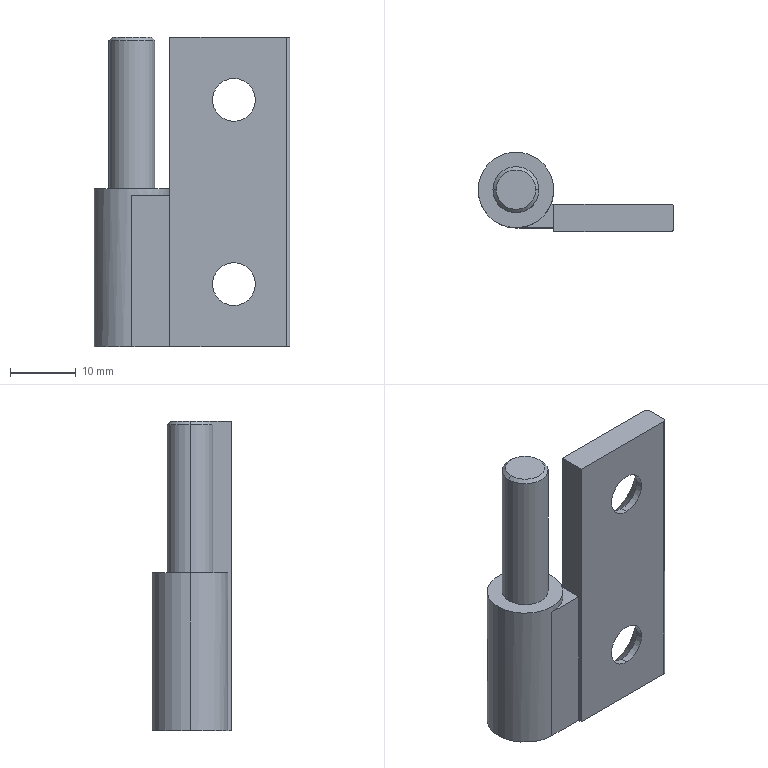Part | SolidWorks | features BaseBody 1 | 1 solid | 31 faces | box 29.75 x 12.05 x 47 mm | volume 6528 mm3 | cylinder 12 | plane 11 | cone 8 | commonest cylinder face diameters 6.5 x4 7 x4 1 x2 11.5 x2
STEP:
#1=CARTESIAN_POINT('',(-3.,6.3,-23.5));
#2=VERTEX_POINT('',#1);
#3=CARTESIAN_POINT('',(3.,6.3,-23.5));
#4=VERTEX_POINT('',#3);
#5=CARTESIAN_POINT('',(0.,6.3,-23.5));
#6=DIRECTION('',(0.,0.,1.));
#7=DIRECTION('',(1.,0.,0.));
#8=AXIS2_PLACEMENT_3D('',#5,#6,#7);
#9=CIRCLE('',#8,3.);
#10=EDGE_CURVE('',#2,#4,#9,.T.);
#11=ORIENTED_EDGE('',*,*,#10,.T.);
#12=CARTESIAN_POINT('',(3.5,6.3,-23.));
#13=VERTEX_POINT('',#12);
#14=CARTESIAN_POINT('',(3.5,6.3,-23.));
#15=DIRECTION('',(0.7071,-0.000000001,0.7071));
#16=VECTOR('',#15,1000.);
#17=LINE('',#14,#16);
#18=EDGE_CURVE('',#4,#13,#17,.T.);
#19=ORIENTED_EDGE('',*,*,#18,.T.);
#20=CARTESIAN_POINT('',(-3.5,6.3,-23.));
#21=VERTEX_POINT('',#20);
#22=CARTESIAN_POINT('',(0.,6.3,-23.));
#23=DIRECTION('',(0.,0.,1.));
#24=DIRECTION('',(-1.,0.,0.));
#25=AXIS2_PLACEMENT_3D('',#22,#23,#24);
#26=CIRCLE('',#25,3.5);
#27=EDGE_CURVE('',#21,#13,#26,.T.);
#28=ORIENTED_EDGE('',*,*,#27,.F.);
#29=CARTESIAN_POINT('',(-3.5,6.3,-23.));
#30=DIRECTION('',(-0.7071,0.000000001,0.7071));
#31=VECTOR('',#30,1000.);
#32=LINE('',#29,#31);
#33=EDGE_CURVE('',#2,#21,#32,.T.);
#34=ORIENTED_EDGE('',*,*,#33,.F.);
#35=EDGE_LOOP('',(#11,#19,#28,#34));
#36=FACE_OUTER_BOUND('',#35,.T.);
#37=CARTESIAN_POINT('',(0.,6.3,-23.));
#38=DIRECTION('',(0.,0.,1.));
#39=DIRECTION('',(-1.,0.000000001,0.));
#40=AXIS2_PLACEMENT_3D('',#37,#38,#39);
#41=CONICAL_SURFACE('',#40,3.5,0.7854);
#42=ADVANCED_FACE('',(#36),#41,.T.);
#43=CARTESIAN_POINT('',(-3.5,6.3,0.5));
#44=VERTEX_POINT('',#43);
#45=CARTESIAN_POINT('',(3.5,6.3,0.5));
#46=VERTEX_POINT('',#45);
#47=CARTESIAN_POINT('',(0.,6.3,0.5));
#48=DIRECTION('',(0.,0.,1.));
#49=DIRECTION('',(1.,0.,0.));
#50=AXIS2_PLACEMENT_3D('',#47,#48,#49);
#51=CIRCLE('',#50,3.5);
#52=EDGE_CURVE('',#44,#46,#51,.T.);
#53=ORIENTED_EDGE('',*,*,#52,.T.);
#54=CARTESIAN_POINT('',(3.5,6.3,23.));
#55=VERTEX_POINT('',#54);
#56=CARTESIAN_POINT('',(3.5,6.3,23.5));
#57=DIRECTION('',(0.,0.,1.));
#58=VECTOR('',#57,1000.);
#59=LINE('',#56,#58);
#60=EDGE_CURVE('',#46,#55,#59,.T.);
#61=ORIENTED_EDGE('',*,*,#60,.T.);
#62=CARTESIAN_POINT('',(-3.5,6.3,23.));
#63=VERTEX_POINT('',#62);
#64=CARTESIAN_POINT('',(0.,6.3,23.));
#65=DIRECTION('',(0.,0.,1.));
#66=DIRECTION('',(-1.,0.,0.));
#67=AXIS2_PLACEMENT_3D('',#64,#65,#66);
#68=CIRCLE('',#67,3.5);
#69=EDGE_CURVE('',#63,#55,#68,.T.);
#70=ORIENTED_EDGE('',*,*,#69,.F.);
#71=CARTESIAN_POINT('',(-3.5,6.3,23.5));
#72=DIRECTION('',(0.,0.,1.));
#73=VECTOR('',#72,1000.);
#74=LINE('',#71,#73);
#75=EDGE_CURVE('',#44,#63,#74,.T.);
#76=ORIENTED_EDGE('',*,*,#75,.F.);
#77=EDGE_LOOP('',(#53,#61,#70,#76));
#78=FACE_OUTER_BOUND('',#77,.T.);
#79=CARTESIAN_POINT('',(0.,6.3,23.5));
#80=DIRECTION('',(0.,0.,1.));
#81=DIRECTION('',(-1.,0.000000142,0.));
#82=AXIS2_PLACEMENT_3D('',#79,#80,#81);
#83=CYLINDRICAL_SURFACE('',#82,3.5);
#84=ADVANCED_FACE('',(#78),#83,.T.);
#85=CARTESIAN_POINT('',(-3.,6.3,23.5));
#86=VERTEX_POINT('',#85);
#87=CARTESIAN_POINT('',(3.,6.3,23.5));
#88=VERTEX_POINT('',#87);
#89=CARTESIAN_POINT('',(0.,6.3,23.5));
#90=DIRECTION('',(0.,0.,1.));
#91=DIRECTION('',(-1.,0.,0.));
#92=AXIS2_PLACEMENT_3D('',#89,#90,#91);
#93=CIRCLE('',#92,3.);
#94=EDGE_CURVE('',#86,#88,#93,.T.);
#95=ORIENTED_EDGE('',*,*,#94,.F.);
#96=CARTESIAN_POINT('',(-3.5,6.3,23.));
#97=DIRECTION('',(-0.7071,0.,-0.7071));
#98=VECTOR('',#97,1000.);
#99=LINE('',#96,#98);
#100=EDGE_CURVE('',#86,#63,#99,.T.);
#101=ORIENTED_EDGE('',*,*,#100,.T.);
#102=ORIENTED_EDGE('',*,*,#69,.T.);
#103=CARTESIAN_POINT('',(3.5,6.3,23.));
#104=DIRECTION('',(0.7071,0.,-0.7071));
#105=VECTOR('',#104,1000.);
#106=LINE('',#103,#105);
#107=EDGE_CURVE('',#88,#55,#106,.T.);
#108=ORIENTED_EDGE('',*,*,#107,.F.);
#109=EDGE_LOOP('',(#95,#101,#102,#108));
#110=FACE_OUTER_BOUND('',#109,.T.);
#111=CARTESIAN_POINT('',(0.,6.3,23.));
#112=DIRECTION('',(0.,0.,-1.));
#113=DIRECTION('',(1.,0.,0.));
#114=AXIS2_PLACEMENT_3D('',#111,#112,#113);
#115=CONICAL_SURFACE('',#114,3.5,0.7854);
#116=ADVANCED_FACE('',(#110),#115,.T.);
#117=CARTESIAN_POINT('',(15.5,1.1,10.75));
#118=VERTEX_POINT('',#117);
#119=CARTESIAN_POINT('',(15.5,1.1,17.25));
#120=VERTEX_POINT('',#119);
#121=CARTESIAN_POINT('',(15.5,1.1,14.));
#122=DIRECTION('',(0.,-1.,0.));
#123=DIRECTION('',(0.,0.,1.));
#124=AXIS2_PLACEMENT_3D('',#121,#122,#123);
#125=CIRCLE('',#124,3.25);
#126=EDGE_CURVE('',#118,#120,#125,.T.);
#127=ORIENTED_EDGE('',*,*,#126,.F.);
#128=CARTESIAN_POINT('',(15.5,0.,10.75));
#129=VERTEX_POINT('',#128);
#130=CARTESIAN_POINT('',(15.5,0.,10.75));
#131=DIRECTION('',(0.,-1.,0.));
#132=VECTOR('',#131,1000.);
#133=LINE('',#130,#132);
#134=EDGE_CURVE('',#118,#129,#133,.T.);
#135=ORIENTED_EDGE('',*,*,#134,.T.);
#136=CARTESIAN_POINT('',(15.5,0.,17.25));
#137=VERTEX_POINT('',#136);
#138=CARTESIAN_POINT('',(15.5,0.,14.));
#139=DIRECTION('',(0.,-1.,0.));
#140=DIRECTION('',(0.,0.,-1.));
#141=AXIS2_PLACEMENT_3D('',#138,#139,#140);
#142=CIRCLE('',#141,3.25);
#143=EDGE_CURVE('',#129,#137,#142,.T.);
#144=ORIENTED_EDGE('',*,*,#143,.T.);
#145=CARTESIAN_POINT('',(15.5,0.,17.25));
#146=DIRECTION('',(0.,-1.,0.));
#147=VECTOR('',#146,1000.);
#148=LINE('',#145,#147);
#149=EDGE_CURVE('',#120,#137,#148,.T.);
#150=ORIENTED_EDGE('',*,*,#149,.F.);
#151=EDGE_LOOP('',(#127,#135,#144,#150));
#152=FACE_OUTER_BOUND('',#151,.T.);
#153=CARTESIAN_POINT('',(15.5,0.,14.));
#154=DIRECTION('',(0.,-1.,0.));
#155=DIRECTION('',(0.000000142,0.,1.));
#156=AXIS2_PLACEMENT_3D('',#153,#154,#155);
#157=CYLINDRICAL_SURFACE('',#156,3.25);
#158=ADVANCED_FACE('',(#152),#157,.F.);
#159=ORIENTED_EDGE('',*,*,#126,.T.);
#160=CARTESIAN_POINT('',(15.5,4.1,20.25));
#161=VERTEX_POINT('',#160);
#162=CARTESIAN_POINT('',(15.5,4.1,20.25));
#163=DIRECTION('',(0.,0.7071,0.7071));
#164=VECTOR('',#163,1000.);
#165=LINE('',#162,#164);
#166=EDGE_CURVE('',#120,#161,#165,.T.);
#167=ORIENTED_EDGE('',*,*,#166,.T.);
#168=CARTESIAN_POINT('',(15.5,4.1,7.75));
#169=VERTEX_POINT('',#168);
#170=CARTESIAN_POINT('',(15.5,4.1,14.));
#171=DIRECTION('',(0.,-1.,0.));
#172=DIRECTION('',(-0.000000001,0.,1.));
#173=AXIS2_PLACEMENT_3D('',#170,#171,#172);
#174=CIRCLE('',#173,6.25);
#175=EDGE_CURVE('',#169,#161,#174,.T.);
#176=ORIENTED_EDGE('',*,*,#175,.F.);
#177=CARTESIAN_POINT('',(15.5,4.1,7.75));
#178=DIRECTION('',(0.,0.7071,-0.7071));
#179=VECTOR('',#178,1000.);
#180=LINE('',#177,#179);
#181=EDGE_CURVE('',#118,#169,#180,.T.);
#182=ORIENTED_EDGE('',*,*,#181,.F.);
#183=EDGE_LOOP('',(#159,#167,#176,#182));
#184=FACE_OUTER_BOUND('',#183,.T.);
#185=CARTESIAN_POINT('',(15.5,4.1,14.));
#186=DIRECTION('',(0.,1.,0.));
#187=DIRECTION('',(0.,0.,-1.));
#188=AXIS2_PLACEMENT_3D('',#185,#186,#187);
#189=CONICAL_SURFACE('',#188,6.25,0.7854);
#190=ADVANCED_FACE('',(#184),#189,.F.);
#191=CARTESIAN_POINT('',(15.5,1.1,-17.25));
#192=VERTEX_POINT('',#191);
#193=CARTESIAN_POINT('',(15.5,1.1,-10.75));
#194=VERTEX_POINT('',#193);
#195=CARTESIAN_POINT('',(15.5,1.1,-14.));
#196=DIRECTION('',(0.,-1.,0.));
#197=DIRECTION('',(0.,0.,1.));
#198=AXIS2_PLACEMENT_3D('',#195,#196,#197);
#199=CIRCLE('',#198,3.25);
#200=EDGE_CURVE('',#192,#194,#199,.T.);
#201=ORIENTED_EDGE('',*,*,#200,.F.);
#202=CARTESIAN_POINT('',(15.5,0.,-17.25));
#203=VERTEX_POINT('',#202);
#204=CARTESIAN_POINT('',(15.5,0.,-17.25));
#205=DIRECTION('',(0.,-1.,0.));
#206=VECTOR('',#205,1000.);
#207=LINE('',#204,#206);
#208=EDGE_CURVE('',#192,#203,#207,.T.);
#209=ORIENTED_EDGE('',*,*,#208,.T.);
#210=CARTESIAN_POINT('',(15.5,0.,-10.75));
#211=VERTEX_POINT('',#210);
#212=CARTESIAN_POINT('',(15.5,0.,-14.));
#213=DIRECTION('',(0.,-1.,0.));
#214=DIRECTION('',(0.,0.,-1.));
#215=AXIS2_PLACEMENT_3D('',#212,#213,#214);
#216=CIRCLE('',#215,3.25);
#217=EDGE_CURVE('',#203,#211,#216,.T.);
#218=ORIENTED_EDGE('',*,*,#217,.T.);
#219=CARTESIAN_POINT('',(15.5,0.,-10.75));
#220=DIRECTION('',(0.,-1.,0.));
#221=VECTOR('',#220,1000.);
#222=LINE('',#219,#221);
#223=EDGE_CURVE('',#194,#211,#222,.T.);
#224=ORIENTED_EDGE('',*,*,#223,.F.);
#225=EDGE_LOOP('',(#201,#209,#218,#224));
#226=FACE_OUTER_BOUND('',#225,.T.);
#227=CARTESIAN_POINT('',(15.5,0.,-14.));
#228=DIRECTION('',(0.,-1.,0.));
#229=DIRECTION('',(0.,0.,1.));
#230=AXIS2_PLACEMENT_3D('',#227,#228,#229);
#231=CYLINDRICAL_SURFACE('',#230,3.25);
#232=ADVANCED_FACE('',(#226),#231,.F.);
#233=ORIENTED_EDGE('',*,*,#200,.T.);
#234=CARTESIAN_POINT('',(15.5,4.1,-7.75));
#235=VERTEX_POINT('',#234);
#236=CARTESIAN_POINT('',(15.5,4.1,-7.75));
#237=DIRECTION('',(0.,0.7071,0.7071));
#238=VECTOR('',#237,1000.);
#239=LINE('',#236,#238);
#240=EDGE_CURVE('',#194,#235,#239,.T.);
#241=ORIENTED_EDGE('',*,*,#240,.T.);
#242=CARTESIAN_POINT('',(15.5,4.1,-20.25));
#243=VERTEX_POINT('',#242);
#244=CARTESIAN_POINT('',(15.5,4.1,-14.));
#245=DIRECTION('',(0.,-1.,0.));
#246=DIRECTION('',(0.,0.,1.));
#247=AXIS2_PLACEMENT_3D('',#244,#245,#246);
#248=CIRCLE('',#247,6.25);
#249=EDGE_CURVE('',#243,#235,#248,.T.);
#250=ORIENTED_EDGE('',*,*,#249,.F.);
#251=CARTESIAN_POINT('',(15.5,4.1,-20.25));
#252=DIRECTION('',(0.,0.7071,-0.7071));
#253=VECTOR('',#252,1000.);
#254=LINE('',#251,#253);
#255=EDGE_CURVE('',#192,#243,#254,.T.);
#256=ORIENTED_EDGE('',*,*,#255,.F.);
#257=EDGE_LOOP('',(#233,#241,#250,#256));
#258=FACE_OUTER_BOUND('',#257,.T.);
#259=CARTESIAN_POINT('',(15.5,4.1,-14.));
#260=DIRECTION('',(0.,1.,0.));
#261=DIRECTION('',(0.,0.,-1.));
#262=AXIS2_PLACEMENT_3D('',#259,#260,#261);
#263=CONICAL_SURFACE('',#262,6.25,0.7854);
#264=ADVANCED_FACE('',(#258),#263,.F.);
#265=CARTESIAN_POINT('',(-5.75,6.3,0.5));
#266=VERTEX_POINT('',#265);
#267=CARTESIAN_POINT('',(5.75,6.3,0.5));
#268=VERTEX_POINT('',#267);
#269=CARTESIAN_POINT('',(0.,6.3,0.5));
#270=DIRECTION('',(0.,0.,1.));
#271=DIRECTION('',(-1.,0.,0.));
#272=AXIS2_PLACEMENT_3D('',#269,#270,#271);
#273=CIRCLE('',#272,5.75);
#274=EDGE_CURVE('',#266,#268,#273,.T.);
#275=ORIENTED_EDGE('',*,*,#274,.F.);
#276=CARTESIAN_POINT('',(-5.75,6.3,-23.5));
#277=VERTEX_POINT('',#276);
#278=CARTESIAN_POINT('',(-5.75,6.3,23.5));
#279=DIRECTION('',(0.,0.,-1.));
#280=VECTOR('',#279,1000.);
#281=LINE('',#278,#280);
#282=EDGE_CURVE('',#266,#277,#281,.T.);
#283=ORIENTED_EDGE('',*,*,#282,.T.);
#284=CARTESIAN_POINT('',(0.,0.55,-23.5));
#285=VERTEX_POINT('',#284);
#286=CARTESIAN_POINT('',(0.,6.3,-23.5));
#287=DIRECTION('',(0.,0.,1.));
#288=DIRECTION('',(1.,0.,0.));
#289=AXIS2_PLACEMENT_3D('',#286,#287,#288);
#290=CIRCLE('',#289,5.75);
#291=EDGE_CURVE('',#277,#285,#290,.T.);
#292=ORIENTED_EDGE('',*,*,#291,.T.);
#293=CARTESIAN_POINT('',(0.,0.55,-0.5));
#294=VERTEX_POINT('',#293);
#295=CARTESIAN_POINT('',(0.,0.55,-0.5));
#296=DIRECTION('',(0.,0.,-1.));
#297=VECTOR('',#296,1000.);
#298=LINE('',#295,#297);
#299=EDGE_CURVE('',#294,#285,#298,.T.);
#300=ORIENTED_EDGE('',*,*,#299,.F.);
#301=CARTESIAN_POINT('',(5.312,4.1,-0.5));
#302=VERTEX_POINT('',#301);
#303=CARTESIAN_POINT('',(0.,6.3,-0.5));
#304=DIRECTION('',(0.,0.,1.));
#305=DIRECTION('',(0.9239,-0.3826,0.));
#306=AXIS2_PLACEMENT_3D('',#303,#304,#305);
#307=CIRCLE('',#306,5.75);
#308=EDGE_CURVE('',#294,#302,#307,.T.);
#309=ORIENTED_EDGE('',*,*,#308,.T.);
#310=CARTESIAN_POINT('',(5.312,4.1,-23.5));
#311=VERTEX_POINT('',#310);
#312=CARTESIAN_POINT('',(5.312,4.1,-23.5));
#313=DIRECTION('',(0.,0.,-1.));
#314=VECTOR('',#313,1000.);
#315=LINE('',#312,#314);
#316=EDGE_CURVE('',#302,#311,#315,.T.);
#317=ORIENTED_EDGE('',*,*,#316,.T.);
#318=CARTESIAN_POINT('',(5.75,6.3,-23.5));
#319=VERTEX_POINT('',#318);
#320=CARTESIAN_POINT('',(0.,6.3,-23.5));
#321=DIRECTION('',(0.,0.,1.));
#322=DIRECTION('',(1.,0.,0.));
#323=AXIS2_PLACEMENT_3D('',#320,#321,#322);
#324=CIRCLE('',#323,5.75);
#325=EDGE_CURVE('',#311,#319,#324,.T.);
#326=ORIENTED_EDGE('',*,*,#325,.T.);
#327=CARTESIAN_POINT('',(5.75,6.3,23.5));
#328=DIRECTION('',(0.,0.,-1.));
#329=VECTOR('',#328,1000.);
#330=LINE('',#327,#329);
#331=EDGE_CURVE('',#268,#319,#330,.T.);
#332=ORIENTED_EDGE('',*,*,#331,.F.);
#333=EDGE_LOOP('',(#275,#283,#292,#300,#309,#317,#326,#332));
#334=FACE_OUTER_BOUND('',#333,.T.);
#335=CARTESIAN_POINT('',(0.,6.3,23.5));
#336=DIRECTION('',(0.,0.,-1.));
#337=DIRECTION('',(1.,0.000000001,0.));
#338=AXIS2_PLACEMENT_3D('',#335,#336,#337);
#339=CYLINDRICAL_SURFACE('',#338,5.75);
#340=ADVANCED_FACE('',(#334),#339,.T.);
#341=CARTESIAN_POINT('',(0.,6.3,-23.));
#342=DIRECTION('',(0.,0.,1.));
#343=DIRECTION('',(-1.,0.,0.));
#344=AXIS2_PLACEMENT_3D('',#341,#342,#343);
#345=CIRCLE('',#344,3.5);
#346=EDGE_CURVE('',#13,#21,#345,.T.);
#347=ORIENTED_EDGE('',*,*,#346,.T.);
#348=CARTESIAN_POINT('',(-3.5,6.3,-23.5));
#349=VERTEX_POINT('',#348);
#350=CARTESIAN_POINT('',(-3.5,6.3,23.5));
#351=DIRECTION('',(0.,0.,-1.));
#352=VECTOR('',#351,1000.);
#353=LINE('',#350,#352);
#354=EDGE_CURVE('',#21,#349,#353,.T.);
#355=ORIENTED_EDGE('',*,*,#354,.T.);
#356=CARTESIAN_POINT('',(3.5,6.3,-23.5));
#357=VERTEX_POINT('',#356);
#358=CARTESIAN_POINT('',(0.,6.3,-23.5));
#359=DIRECTION('',(0.,0.,1.));
#360=DIRECTION('',(-1.,-0.000000142,0.));
#361=AXIS2_PLACEMENT_3D('',#358,#359,#360);
#362=CIRCLE('',#361,3.5);
#363=EDGE_CURVE('',#357,#349,#362,.T.);
#364=ORIENTED_EDGE('',*,*,#363,.F.);
#365=CARTESIAN_POINT('',(3.5,6.3,23.5));
#366=DIRECTION('',(0.,0.,-1.));
#367=VECTOR('',#366,1000.);
#368=LINE('',#365,#367);
#369=EDGE_CURVE('',#13,#357,#368,.T.);
#370=ORIENTED_EDGE('',*,*,#369,.F.);
#371=EDGE_LOOP('',(#347,#355,#364,#370));
#372=FACE_OUTER_BOUND('',#371,.T.);
#373=CARTESIAN_POINT('',(0.,6.3,23.5));
#374=DIRECTION('',(0.,0.,-1.));
#375=DIRECTION('',(1.,0.,0.));
#376=AXIS2_PLACEMENT_3D('',#373,#374,#375);
#377=CYLINDRICAL_SURFACE('',#376,3.5);
#378=ADVANCED_FACE('',(#372),#377,.F.);
#379=CARTESIAN_POINT('',(5.75,4.1,-0.5));
#380=VERTEX_POINT('',#379);
#381=CARTESIAN_POINT('',(5.75,4.1,-0.5));
#382=DIRECTION('',(-1.,0.,0.));
#383=VECTOR('',#382,1000.);
#384=LINE('',#381,#383);
#385=EDGE_CURVE('',#380,#302,#384,.T.);
#386=ORIENTED_EDGE('',*,*,#385,.T.);
#387=ORIENTED_EDGE('',*,*,#308,.F.);
#388=CARTESIAN_POINT('',(5.75,0.55,-0.5));
#389=VERTEX_POINT('',#388);
#390=CARTESIAN_POINT('',(0.,0.55,-0.5));
#391=DIRECTION('',(1.,0.,0.));
#392=VECTOR('',#391,1000.);
#393=LINE('',#390,#392);
#394=EDGE_CURVE('',#294,#389,#393,.T.);
#395=ORIENTED_EDGE('',*,*,#394,.T.);
#396=CARTESIAN_POINT('',(5.75,0.55,-0.5));
#397=DIRECTION('',(0.,-1.,0.));
#398=VECTOR('',#397,1000.);
#399=LINE('',#396,#398);
#400=EDGE_CURVE('',#380,#389,#399,.T.);
#401=ORIENTED_EDGE('',*,*,#400,.F.);
#402=EDGE_LOOP('',(#386,#387,#395,#401));
#403=FACE_OUTER_BOUND('',#402,.T.);
#404=CARTESIAN_POINT('',(0.,0.55,-0.5));
#405=DIRECTION('',(0.,0.,1.));
#406=DIRECTION('',(1.,0.,0.));
#407=AXIS2_PLACEMENT_3D('',#404,#405,#406);
#408=PLANE('',#407);
#409=ADVANCED_FACE('',(#403),#408,.T.);
#410=CARTESIAN_POINT('',(5.75,4.1,23.5));
#411=VERTEX_POINT('',#410);
#412=CARTESIAN_POINT('',(5.75,4.1,-0.5));
#413=DIRECTION('',(0.,0.,-1.));
#414=VECTOR('',#413,1000.);
#415=LINE('',#412,#414);
#416=EDGE_CURVE('',#411,#380,#415,.T.);
#417=ORIENTED_EDGE('',*,*,#416,.F.);
#418=CARTESIAN_POINT('',(23.5,4.1,23.5));
#419=VERTEX_POINT('',#418);
#420=CARTESIAN_POINT('',(5.75,4.1,23.5));
#421=DIRECTION('',(-1.,0.,0.));
#422=VECTOR('',#421,1000.);
#423=LINE('',#420,#422);
#424=EDGE_CURVE('',#419,#411,#423,.T.);
#425=ORIENTED_EDGE('',*,*,#424,.F.);
#426=CARTESIAN_POINT('',(23.5,4.1,-23.5));
#427=VERTEX_POINT('',#426);
#428=CARTESIAN_POINT('',(23.5,4.1,23.5));
#429=DIRECTION('',(0.,0.,-1.));
#430=VECTOR('',#429,1000.);
#431=LINE('',#428,#430);
#432=EDGE_CURVE('',#419,#427,#431,.T.);
#433=ORIENTED_EDGE('',*,*,#432,.T.);
#434=CARTESIAN_POINT('',(23.5,4.1,-23.5));
#435=DIRECTION('',(-1.,0.,0.));
#436=VECTOR('',#435,1000.);
#437=LINE('',#434,#436);
#438=EDGE_CURVE('',#427,#311,#437,.T.);
#439=ORIENTED_EDGE('',*,*,#438,.T.);
#440=ORIENTED_EDGE('',*,*,#316,.F.);
#441=ORIENTED_EDGE('',*,*,#385,.F.);
#442=EDGE_LOOP('',(#417,#425,#433,#439,#440,#441));
#443=FACE_OUTER_BOUND('',#442,.T.);
#444=ORIENTED_EDGE('',*,*,#249,.T.);
#445=CARTESIAN_POINT('',(15.5,4.1,-14.));
#446=DIRECTION('',(0.,-1.,0.));
#447=DIRECTION('',(0.,0.,1.));
#448=AXIS2_PLACEMENT_3D('',#445,#446,#447);
#449=CIRCLE('',#448,6.25);
#450=EDGE_CURVE('',#235,#243,#449,.T.);
#451=ORIENTED_EDGE('',*,*,#450,.T.);
#452=EDGE_LOOP('',(#444,#451));
#453=FACE_BOUND('',#452,.T.);
#454=ORIENTED_EDGE('',*,*,#175,.T.);
#455=CARTESIAN_POINT('',(15.5,4.1,14.));
#456=DIRECTION('',(0.,-1.,0.));
#457=DIRECTION('',(-0.000000001,0.,1.));
#458=AXIS2_PLACEMENT_3D('',#455,#456,#457);
#459=CIRCLE('',#458,6.25);
#460=EDGE_CURVE('',#161,#169,#459,.T.);
#461=ORIENTED_EDGE('',*,*,#460,.T.);
#462=EDGE_LOOP('',(#454,#461));
#463=FACE_BOUND('',#462,.T.);
#464=CARTESIAN_POINT('',(5.312,4.1,23.5));
#465=DIRECTION('',(0.,1.,0.));
#466=DIRECTION('',(1.,0.,0.));
#467=AXIS2_PLACEMENT_3D('',#464,#465,#466);
#468=PLANE('',#467);
#469=ADVANCED_FACE('',(#443,#453,#463),#468,.T.);
#470=ORIENTED_EDGE('',*,*,#394,.F.);
#471=ORIENTED_EDGE('',*,*,#299,.T.);
#472=CARTESIAN_POINT('',(5.75,0.55,-23.5));
#473=VERTEX_POINT('',#472);
#474=CARTESIAN_POINT('',(0.,0.55,-23.5));
#475=DIRECTION('',(1.,0.,0.));
#476=VECTOR('',#475,1000.);
#477=LINE('',#474,#476);
#478=EDGE_CURVE('',#285,#473,#477,.T.);
#479=ORIENTED_EDGE('',*,*,#478,.T.);
#480=CARTESIAN_POINT('',(5.75,0.55,-23.5));
#481=DIRECTION('',(0.,0.,-1.));
#482=VECTOR('',#481,1000.);
#483=LINE('',#480,#482);
#484=EDGE_CURVE('',#389,#473,#483,.T.);
#485=ORIENTED_EDGE('',*,*,#484,.F.);
#486=EDGE_LOOP('',(#470,#471,#479,#485));
#487=FACE_OUTER_BOUND('',#486,.T.);
#488=CARTESIAN_POINT('',(0.,0.55,-23.5));
#489=DIRECTION('',(0.,-1.,0.));
#490=DIRECTION('',(1.,0.,0.));
#491=AXIS2_PLACEMENT_3D('',#488,#489,#490);
#492=PLANE('',#491);
#493=ADVANCED_FACE('',(#487),#492,.T.);
#494=ORIENTED_EDGE('',*,*,#424,.T.);
#495=CARTESIAN_POINT('',(5.75,0.,23.5));
#496=VERTEX_POINT('',#495);
#497=CARTESIAN_POINT('',(5.75,4.1,23.5));
#498=DIRECTION('',(0.,-1.,0.));
#499=VECTOR('',#498,1000.);
#500=LINE('',#497,#499);
#501=EDGE_CURVE('',#411,#496,#500,.T.);
#502=ORIENTED_EDGE('',*,*,#501,.T.);
#503=CARTESIAN_POINT('',(23.5,0.,23.5));
#504=VERTEX_POINT('',#503);
#505=CARTESIAN_POINT('',(5.75,0.,23.5));
#506=DIRECTION('',(1.,0.,0.));
#507=VECTOR('',#506,1000.);
#508=LINE('',#505,#507);
#509=EDGE_CURVE('',#496,#504,#508,.T.);
#510=ORIENTED_EDGE('',*,*,#509,.T.);
#511=CARTESIAN_POINT('',(24.,0.5,23.5));
#512=VERTEX_POINT('',#511);
#513=CARTESIAN_POINT('',(23.5,0.5,23.5));
#514=DIRECTION('',(0.,0.,1.));
#515=DIRECTION('',(0.,-1.,0.));
#516=AXIS2_PLACEMENT_3D('',#513,#514,#515);
#517=CIRCLE('',#516,0.5);
#518=EDGE_CURVE('',#504,#512,#517,.T.);
#519=ORIENTED_EDGE('',*,*,#518,.T.);
#520=CARTESIAN_POINT('',(24.,3.6,23.5));
#521=VERTEX_POINT('',#520);
#522=CARTESIAN_POINT('',(24.,0.5,23.5));
#523=DIRECTION('',(0.,1.,0.));
#524=VECTOR('',#523,1000.);
#525=LINE('',#522,#524);
#526=EDGE_CURVE('',#512,#521,#525,.T.);
#527=ORIENTED_EDGE('',*,*,#526,.T.);
#528=CARTESIAN_POINT('',(23.5,3.6,23.5));
#529=DIRECTION('',(0.,0.,1.));
#530=DIRECTION('',(1.,0.,0.));
#531=AXIS2_PLACEMENT_3D('',#528,#529,#530);
#532=CIRCLE('',#531,0.5);
#533=EDGE_CURVE('',#521,#419,#532,.T.);
#534=ORIENTED_EDGE('',*,*,#533,.T.);
#535=EDGE_LOOP('',(#494,#502,#510,#519,#527,#534));
#536=FACE_OUTER_BOUND('',#535,.T.);
#537=CARTESIAN_POINT('',(5.75,0.,23.5));
#538=DIRECTION('',(0.,0.,1.));
#539=DIRECTION('',(1.,0.,0.));
#540=AXIS2_PLACEMENT_3D('',#537,#538,#539);
#541=PLANE('',#540);
#542=ADVANCED_FACE('',(#536),#541,.T.);
#543=ORIENTED_EDGE('',*,*,#501,.F.);
#544=ORIENTED_EDGE('',*,*,#416,.T.);
#545=ORIENTED_EDGE('',*,*,#400,.T.);
#546=ORIENTED_EDGE('',*,*,#484,.T.);
#547=CARTESIAN_POINT('',(5.75,0.,-23.5));
#548=VERTEX_POINT('',#547);
#549=CARTESIAN_POINT('',(5.75,0.55,-23.5));
#550=DIRECTION('',(0.,-1.,0.));
#551=VECTOR('',#550,1000.);
#552=LINE('',#549,#551);
#553=EDGE_CURVE('',#473,#548,#552,.T.);
#554=ORIENTED_EDGE('',*,*,#553,.T.);
#555=CARTESIAN_POINT('',(5.75,0.,-23.5));
#556=DIRECTION('',(0.,0.,-1.));
#557=VECTOR('',#556,1000.);
#558=LINE('',#555,#557);
#559=EDGE_CURVE('',#496,#548,#558,.T.);
#560=ORIENTED_EDGE('',*,*,#559,.F.);
#561=EDGE_LOOP('',(#543,#544,#545,#546,#554,#560));
#562=FACE_OUTER_BOUND('',#561,.T.);
#563=CARTESIAN_POINT('',(5.75,0.,23.5));
#564=DIRECTION('',(-1.,0.,0.));
#565=DIRECTION('',(0.,1.,0.));
#566=AXIS2_PLACEMENT_3D('',#563,#564,#565);
#567=PLANE('',#566);
#568=ADVANCED_FACE('',(#562),#567,.T.);
#569=CARTESIAN_POINT('',(23.5,0.,-23.5));
#570=VERTEX_POINT('',#569);
#571=CARTESIAN_POINT('',(5.75,0.,-23.5));
#572=DIRECTION('',(1.,0.,0.));
#573=VECTOR('',#572,1000.);
#574=LINE('',#571,#573);
#575=EDGE_CURVE('',#548,#570,#574,.T.);
#576=ORIENTED_EDGE('',*,*,#575,.T.);
#577=CARTESIAN_POINT('',(23.5,0.,-23.5));
#578=DIRECTION('',(0.,0.,-1.));
#579=VECTOR('',#578,1000.);
#580=LINE('',#577,#579);
#581=EDGE_CURVE('',#504,#570,#580,.T.);
#582=ORIENTED_EDGE('',*,*,#581,.F.);
#583=ORIENTED_EDGE('',*,*,#509,.F.);
#584=ORIENTED_EDGE('',*,*,#559,.T.);
#585=EDGE_LOOP('',(#576,#582,#583,#584));
#586=FACE_OUTER_BOUND('',#585,.T.);
#587=CARTESIAN_POINT('',(15.5,0.,-14.));
#588=DIRECTION('',(0.,-1.,0.));
#589=DIRECTION('',(0.,0.,-1.));
#590=AXIS2_PLACEMENT_3D('',#587,#588,#589);
#591=CIRCLE('',#590,3.25);
#592=EDGE_CURVE('',#211,#203,#591,.T.);
#593=ORIENTED_EDGE('',*,*,#592,.F.);
#594=ORIENTED_EDGE('',*,*,#217,.F.);
#595=EDGE_LOOP('',(#593,#594));
#596=FACE_BOUND('',#595,.T.);
#597=CARTESIAN_POINT('',(15.5,0.,14.));
#598=DIRECTION('',(0.,-1.,0.));
#599=DIRECTION('',(0.,0.,-1.));
#600=AXIS2_PLACEMENT_3D('',#597,#598,#599);
#601=CIRCLE('',#600,3.25);
#602=EDGE_CURVE('',#137,#129,#601,.T.);
#603=ORIENTED_EDGE('',*,*,#602,.F.);
#604=ORIENTED_EDGE('',*,*,#143,.F.);
#605=EDGE_LOOP('',(#603,#604));
#606=FACE_BOUND('',#605,.T.);
#607=CARTESIAN_POINT('',(5.75,0.,-23.5));
#608=DIRECTION('',(0.,-1.,0.));
#609=DIRECTION('',(1.,0.,0.));
#610=AXIS2_PLACEMENT_3D('',#607,#608,#609);
#611=PLANE('',#610);
#612=ADVANCED_FACE('',(#586,#596,#606),#611,.T.);
#613=CARTESIAN_POINT('',(24.,0.5,-23.5));
#614=VERTEX_POINT('',#613);
#615=CARTESIAN_POINT('',(23.5,0.5,-23.5));
#616=DIRECTION('',(0.,0.,1.));
#617=DIRECTION('',(0.,-1.,0.));
#618=AXIS2_PLACEMENT_3D('',#615,#616,#617);
#619=CIRCLE('',#618,0.5);
#620=EDGE_CURVE('',#570,#614,#619,.T.);
#621=ORIENTED_EDGE('',*,*,#620,.T.);
#622=CARTESIAN_POINT('',(24.,0.5,-23.5));
#623=DIRECTION('',(0.,0.,-1.));
#624=VECTOR('',#623,1000.);
#625=LINE('',#622,#624);
#626=EDGE_CURVE('',#512,#614,#625,.T.);
#627=ORIENTED_EDGE('',*,*,#626,.F.);
#628=ORIENTED_EDGE('',*,*,#518,.F.);
#629=ORIENTED_EDGE('',*,*,#581,.T.);
#630=EDGE_LOOP('',(#621,#627,#628,#629));
#631=FACE_OUTER_BOUND('',#630,.T.);
#632=CARTESIAN_POINT('',(23.5,0.5,23.5));
#633=DIRECTION('',(0.,0.,-1.));
#634=DIRECTION('',(1.,0.,0.));
#635=AXIS2_PLACEMENT_3D('',#632,#633,#634);
#636=CYLINDRICAL_SURFACE('',#635,0.5);
#637=ADVANCED_FACE('',(#631),#636,.T.);
#638=CARTESIAN_POINT('',(24.,3.6,-23.5));
#639=VERTEX_POINT('',#638);
#640=CARTESIAN_POINT('',(24.,0.5,-23.5));
#641=DIRECTION('',(0.,1.,0.));
#642=VECTOR('',#641,1000.);
#643=LINE('',#640,#642);
#644=EDGE_CURVE('',#614,#639,#643,.T.);
#645=ORIENTED_EDGE('',*,*,#644,.T.);
#646=CARTESIAN_POINT('',(24.,3.6,-23.5));
#647=DIRECTION('',(0.,0.,-1.));
#648=VECTOR('',#647,1000.);
#649=LINE('',#646,#648);
#650=EDGE_CURVE('',#521,#639,#649,.T.);
#651=ORIENTED_EDGE('',*,*,#650,.F.);
#652=ORIENTED_EDGE('',*,*,#526,.F.);
#653=ORIENTED_EDGE('',*,*,#626,.T.);
#654=EDGE_LOOP('',(#645,#651,#652,#653));
#655=FACE_OUTER_BOUND('',#654,.T.);
#656=CARTESIAN_POINT('',(24.,0.5,-23.5));
#657=DIRECTION('',(1.,0.,0.));
#658=DIRECTION('',(0.,1.,0.));
#659=AXIS2_PLACEMENT_3D('',#656,#657,#658);
#660=PLANE('',#659);
#661=ADVANCED_FACE('',(#655),#660,.T.);
#662=CARTESIAN_POINT('',(23.5,3.6,-23.5));
#663=DIRECTION('',(0.,0.,1.));
#664=DIRECTION('',(1.,0.,0.));
#665=AXIS2_PLACEMENT_3D('',#662,#663,#664);
#666=CIRCLE('',#665,0.5);
#667=EDGE_CURVE('',#639,#427,#666,.T.);
#668=ORIENTED_EDGE('',*,*,#667,.T.);
#669=ORIENTED_EDGE('',*,*,#432,.F.);
#670=ORIENTED_EDGE('',*,*,#533,.F.);
#671=ORIENTED_EDGE('',*,*,#650,.T.);
#672=EDGE_LOOP('',(#668,#669,#670,#671));
#673=FACE_OUTER_BOUND('',#672,.T.);
#674=CARTESIAN_POINT('',(23.5,3.6,23.5));
#675=DIRECTION('',(0.,0.,-1.));
#676=DIRECTION('',(0.,1.,0.));
#677=AXIS2_PLACEMENT_3D('',#674,#675,#676);
#678=CYLINDRICAL_SURFACE('',#677,0.5);
#679=ADVANCED_FACE('',(#673),#678,.T.);
#680=ORIENTED_EDGE('',*,*,#438,.F.);
#681=ORIENTED_EDGE('',*,*,#667,.F.);
#682=ORIENTED_EDGE('',*,*,#644,.F.);
#683=ORIENTED_EDGE('',*,*,#620,.F.);
#684=ORIENTED_EDGE('',*,*,#575,.F.);
#685=ORIENTED_EDGE('',*,*,#553,.F.);
#686=ORIENTED_EDGE('',*,*,#478,.F.);
#687=ORIENTED_EDGE('',*,*,#291,.F.);
#688=CARTESIAN_POINT('',(0.,6.3,-23.5));
#689=DIRECTION('',(0.,0.,1.));
#690=DIRECTION('',(1.,0.,0.));
#691=AXIS2_PLACEMENT_3D('',#688,#689,#690);
#692=CIRCLE('',#691,5.75);
#693=EDGE_CURVE('',#319,#277,#692,.T.);
#694=ORIENTED_EDGE('',*,*,#693,.F.);
#695=ORIENTED_EDGE('',*,*,#325,.F.);
#696=EDGE_LOOP('',(#680,#681,#682,#683,#684,#685,#686,#687,#694,#695));
#697=FACE_OUTER_BOUND('',#696,.T.);
#698=ORIENTED_EDGE('',*,*,#363,.T.);
#699=CARTESIAN_POINT('',(0.,6.3,-23.5));
#700=DIRECTION('',(0.,0.,1.));
#701=DIRECTION('',(-1.,-0.000000142,0.));
#702=AXIS2_PLACEMENT_3D('',#699,#700,#701);
#703=CIRCLE('',#702,3.5);
#704=EDGE_CURVE('',#349,#357,#703,.T.);
#705=ORIENTED_EDGE('',*,*,#704,.T.);
#706=EDGE_LOOP('',(#698,#705));
#707=FACE_BOUND('',#706,.T.);
#708=CARTESIAN_POINT('',(-5.75,0.,-23.5));
#709=DIRECTION('',(0.,0.,-1.));
#710=DIRECTION('',(0.,1.,0.));
#711=AXIS2_PLACEMENT_3D('',#708,#709,#710);
#712=PLANE('',#711);
#713=ADVANCED_FACE('',(#697,#707),#712,.T.);
#714=CARTESIAN_POINT('',(0.,6.3,23.5));
#715=DIRECTION('',(0.,0.,1.));
#716=DIRECTION('',(-1.,0.,0.));
#717=AXIS2_PLACEMENT_3D('',#714,#715,#716);
#718=CIRCLE('',#717,3.);
#719=EDGE_CURVE('',#88,#86,#718,.T.);
#720=ORIENTED_EDGE('',*,*,#719,.T.);
#721=ORIENTED_EDGE('',*,*,#94,.T.);
#722=EDGE_LOOP('',(#720,#721));
#723=FACE_OUTER_BOUND('',#722,.T.);
#724=CARTESIAN_POINT('',(3.,3.3,23.5));
#725=DIRECTION('',(0.,0.,1.));
#726=DIRECTION('',(0.,1.,0.));
#727=AXIS2_PLACEMENT_3D('',#724,#725,#726);
#728=PLANE('',#727);
#729=ADVANCED_FACE('',(#723),#728,.T.);
#730=CARTESIAN_POINT('',(0.,6.3,0.5));
#731=DIRECTION('',(0.,0.,1.));
#732=DIRECTION('',(-1.,0.,0.));
#733=AXIS2_PLACEMENT_3D('',#730,#731,#732);
#734=CIRCLE('',#733,5.75);
#735=EDGE_CURVE('',#268,#266,#734,.T.);
#736=ORIENTED_EDGE('',*,*,#735,.T.);
#737=ORIENTED_EDGE('',*,*,#274,.T.);
#738=EDGE_LOOP('',(#736,#737));
#739=FACE_OUTER_BOUND('',#738,.T.);
#740=ORIENTED_EDGE('',*,*,#52,.F.);
#741=CARTESIAN_POINT('',(0.,6.3,0.5));
#742=DIRECTION('',(0.,0.,1.));
#743=DIRECTION('',(1.,0.,0.));
#744=AXIS2_PLACEMENT_3D('',#741,#742,#743);
#745=CIRCLE('',#744,3.5);
#746=EDGE_CURVE('',#46,#44,#745,.T.);
#747=ORIENTED_EDGE('',*,*,#746,.F.);
#748=EDGE_LOOP('',(#740,#747));
#749=FACE_BOUND('',#748,.T.);
#750=CARTESIAN_POINT('',(5.75,0.3929,0.5));
#751=DIRECTION('',(0.,0.,1.));
#752=DIRECTION('',(0.,1.,0.));
#753=AXIS2_PLACEMENT_3D('',#750,#751,#752);
#754=PLANE('',#753);
#755=ADVANCED_FACE('',(#739,#749),#754,.T.);
#756=ORIENTED_EDGE('',*,*,#10,.F.);
#757=CARTESIAN_POINT('',(0.,6.3,-23.5));
#758=DIRECTION('',(0.,0.,1.));
#759=DIRECTION('',(1.,0.,0.));
#760=AXIS2_PLACEMENT_3D('',#757,#758,#759);
#761=CIRCLE('',#760,3.);
#762=EDGE_CURVE('',#4,#2,#761,.T.);
#763=ORIENTED_EDGE('',*,*,#762,.F.);
#764=EDGE_LOOP('',(#756,#763));
#765=FACE_OUTER_BOUND('',#764,.T.);
#766=CARTESIAN_POINT('',(-3.,3.3,-23.5));
#767=DIRECTION('',(0.,0.,-1.));
#768=DIRECTION('',(0.,1.,0.));
#769=AXIS2_PLACEMENT_3D('',#766,#767,#768);
#770=PLANE('',#769);
#771=ADVANCED_FACE('',(#765),#770,.T.);
#772=ORIENTED_EDGE('',*,*,#354,.F.);
#773=ORIENTED_EDGE('',*,*,#27,.T.);
#774=ORIENTED_EDGE('',*,*,#369,.T.);
#775=ORIENTED_EDGE('',*,*,#704,.F.);
#776=EDGE_LOOP('',(#772,#773,#774,#775));
#777=FACE_OUTER_BOUND('',#776,.T.);
#778=CARTESIAN_POINT('',(0.,6.3,23.5));
#779=DIRECTION('',(0.,0.,-1.));
#780=DIRECTION('',(1.,0.,0.));
#781=AXIS2_PLACEMENT_3D('',#778,#779,#780);
#782=CYLINDRICAL_SURFACE('',#781,3.5);
#783=ADVANCED_FACE('',(#777),#782,.F.);
#784=ORIENTED_EDGE('',*,*,#282,.F.);
#785=ORIENTED_EDGE('',*,*,#735,.F.);
#786=ORIENTED_EDGE('',*,*,#331,.T.);
#787=ORIENTED_EDGE('',*,*,#693,.T.);
#788=EDGE_LOOP('',(#784,#785,#786,#787));
#789=FACE_OUTER_BOUND('',#788,.T.);
#790=CARTESIAN_POINT('',(0.,6.3,23.5));
#791=DIRECTION('',(0.,0.,-1.));
#792=DIRECTION('',(1.,0.000000001,0.));
#793=AXIS2_PLACEMENT_3D('',#790,#791,#792);
#794=CYLINDRICAL_SURFACE('',#793,5.75);
#795=ADVANCED_FACE('',(#789),#794,.T.);
#796=ORIENTED_EDGE('',*,*,#240,.F.);
#797=CARTESIAN_POINT('',(15.5,1.1,-14.));
#798=DIRECTION('',(0.,-1.,0.));
#799=DIRECTION('',(0.,0.,1.));
#800=AXIS2_PLACEMENT_3D('',#797,#798,#799);
#801=CIRCLE('',#800,3.25);
#802=EDGE_CURVE('',#194,#192,#801,.T.);
#803=ORIENTED_EDGE('',*,*,#802,.T.);
#804=ORIENTED_EDGE('',*,*,#255,.T.);
#805=ORIENTED_EDGE('',*,*,#450,.F.);
#806=EDGE_LOOP('',(#796,#803,#804,#805));
#807=FACE_OUTER_BOUND('',#806,.T.);
#808=CARTESIAN_POINT('',(15.5,4.1,-14.));
#809=DIRECTION('',(0.,1.,0.));
#810=DIRECTION('',(0.,0.,-1.));
#811=AXIS2_PLACEMENT_3D('',#808,#809,#810);
#812=CONICAL_SURFACE('',#811,6.25,0.7854);
#813=ADVANCED_FACE('',(#807),#812,.F.);
#814=ORIENTED_EDGE('',*,*,#208,.F.);
#815=ORIENTED_EDGE('',*,*,#802,.F.);
#816=ORIENTED_EDGE('',*,*,#223,.T.);
#817=ORIENTED_EDGE('',*,*,#592,.T.);
#818=EDGE_LOOP('',(#814,#815,#816,#817));
#819=FACE_OUTER_BOUND('',#818,.T.);
#820=CARTESIAN_POINT('',(15.5,0.,-14.));
#821=DIRECTION('',(0.,-1.,0.));
#822=DIRECTION('',(0.,0.,1.));
#823=AXIS2_PLACEMENT_3D('',#820,#821,#822);
#824=CYLINDRICAL_SURFACE('',#823,3.25);
#825=ADVANCED_FACE('',(#819),#824,.F.);
#826=ORIENTED_EDGE('',*,*,#166,.F.);
#827=CARTESIAN_POINT('',(15.5,1.1,14.));
#828=DIRECTION('',(0.,-1.,0.));
#829=DIRECTION('',(0.,0.,1.));
#830=AXIS2_PLACEMENT_3D('',#827,#828,#829);
#831=CIRCLE('',#830,3.25);
#832=EDGE_CURVE('',#120,#118,#831,.T.);
#833=ORIENTED_EDGE('',*,*,#832,.T.);
#834=ORIENTED_EDGE('',*,*,#181,.T.);
#835=ORIENTED_EDGE('',*,*,#460,.F.);
#836=EDGE_LOOP('',(#826,#833,#834,#835));
#837=FACE_OUTER_BOUND('',#836,.T.);
#838=CARTESIAN_POINT('',(15.5,4.1,14.));
#839=DIRECTION('',(0.,1.,0.));
#840=DIRECTION('',(0.,0.,-1.));
#841=AXIS2_PLACEMENT_3D('',#838,#839,#840);
#842=CONICAL_SURFACE('',#841,6.25,0.7854);
#843=ADVANCED_FACE('',(#837),#842,.F.);
#844=ORIENTED_EDGE('',*,*,#134,.F.);
#845=ORIENTED_EDGE('',*,*,#832,.F.);
#846=ORIENTED_EDGE('',*,*,#149,.T.);
#847=ORIENTED_EDGE('',*,*,#602,.T.);
#848=EDGE_LOOP('',(#844,#845,#846,#847));
#849=FACE_OUTER_BOUND('',#848,.T.);
#850=CARTESIAN_POINT('',(15.5,0.,14.));
#851=DIRECTION('',(0.,-1.,0.));
#852=DIRECTION('',(0.000000142,0.,1.));
#853=AXIS2_PLACEMENT_3D('',#850,#851,#852);
#854=CYLINDRICAL_SURFACE('',#853,3.25);
#855=ADVANCED_FACE('',(#849),#854,.F.);
#856=ORIENTED_EDGE('',*,*,#100,.F.);
#857=ORIENTED_EDGE('',*,*,#719,.F.);
#858=ORIENTED_EDGE('',*,*,#107,.T.);
#859=CARTESIAN_POINT('',(0.,6.3,23.));
#860=DIRECTION('',(0.,0.,1.));
#861=DIRECTION('',(-1.,0.,0.));
#862=AXIS2_PLACEMENT_3D('',#859,#860,#861);
#863=CIRCLE('',#862,3.5);
#864=EDGE_CURVE('',#55,#63,#863,.T.);
#865=ORIENTED_EDGE('',*,*,#864,.T.);
#866=EDGE_LOOP('',(#856,#857,#858,#865));
#867=FACE_OUTER_BOUND('',#866,.T.);
#868=CARTESIAN_POINT('',(0.,6.3,23.));
#869=DIRECTION('',(0.,0.,-1.));
#870=DIRECTION('',(1.,0.,0.));
#871=AXIS2_PLACEMENT_3D('',#868,#869,#870);
#872=CONICAL_SURFACE('',#871,3.5,0.7854);
#873=ADVANCED_FACE('',(#867),#872,.T.);
#874=ORIENTED_EDGE('',*,*,#60,.F.);
#875=ORIENTED_EDGE('',*,*,#746,.T.);
#876=ORIENTED_EDGE('',*,*,#75,.T.);
#877=ORIENTED_EDGE('',*,*,#864,.F.);
#878=EDGE_LOOP('',(#874,#875,#876,#877));
#879=FACE_OUTER_BOUND('',#878,.T.);
#880=CARTESIAN_POINT('',(0.,6.3,23.5));
#881=DIRECTION('',(0.,0.,1.));
#882=DIRECTION('',(-1.,0.000000142,0.));
#883=AXIS2_PLACEMENT_3D('',#880,#881,#882);
#884=CYLINDRICAL_SURFACE('',#883,3.5);
#885=ADVANCED_FACE('',(#879),#884,.T.);
#886=ORIENTED_EDGE('',*,*,#18,.F.);
#887=ORIENTED_EDGE('',*,*,#762,.T.);
#888=ORIENTED_EDGE('',*,*,#33,.T.);
#889=ORIENTED_EDGE('',*,*,#346,.F.);
#890=EDGE_LOOP('',(#886,#887,#888,#889));
#891=FACE_OUTER_BOUND('',#890,.T.);
#892=CARTESIAN_POINT('',(0.,6.3,-23.));
#893=DIRECTION('',(0.,0.,1.));
#894=DIRECTION('',(-1.,0.000000001,0.));
#895=AXIS2_PLACEMENT_3D('',#892,#893,#894);
#896=CONICAL_SURFACE('',#895,3.5,0.7854);
#897=ADVANCED_FACE('',(#891),#896,.T.);
#898=CLOSED_SHELL('',(#42,#84,#116,#158,#190,#232,#264,#340,#378,#409,#469,#493,#542,#568,#612,#637,#661,#679,#713,#729,#755,#771,#783,#795,#813,#825,#843,#855,#873,#885,#897));
#899=MANIFOLD_SOLID_BREP('',#898);
#900=CARTESIAN_POINT('',(0.,0.,0.));
#901=DIRECTION('',(0.,0.,1.));
#902=DIRECTION('',(1.,0.,0.));
#903=AXIS2_PLACEMENT_3D('',#900,#901,#902);
#904=(LENGTH_UNIT()NAMED_UNIT(*)SI_UNIT(.MILLI.,.METRE.));
#905=UNCERTAINTY_MEASURE_WITH_UNIT(LENGTH_MEASURE(0.00001),#904,'','');
#906=(NAMED_UNIT(*)PLANE_ANGLE_UNIT()SI_UNIT($,.RADIAN.));
#907=(NAMED_UNIT(*)SI_UNIT($,.STERADIAN.)SOLID_ANGLE_UNIT());
#908=(GEOMETRIC_REPRESENTATION_CONTEXT(3)GLOBAL_UNCERTAINTY_ASSIGNED_CONTEXT((#905))GLOBAL_UNIT_ASSIGNED_CONTEXT((#904,#906,#907))REPRESENTATION_CONTEXT('',''));
#909=ADVANCED_BREP_SHAPE_REPRESENTATION('',(#899,#903),#908);